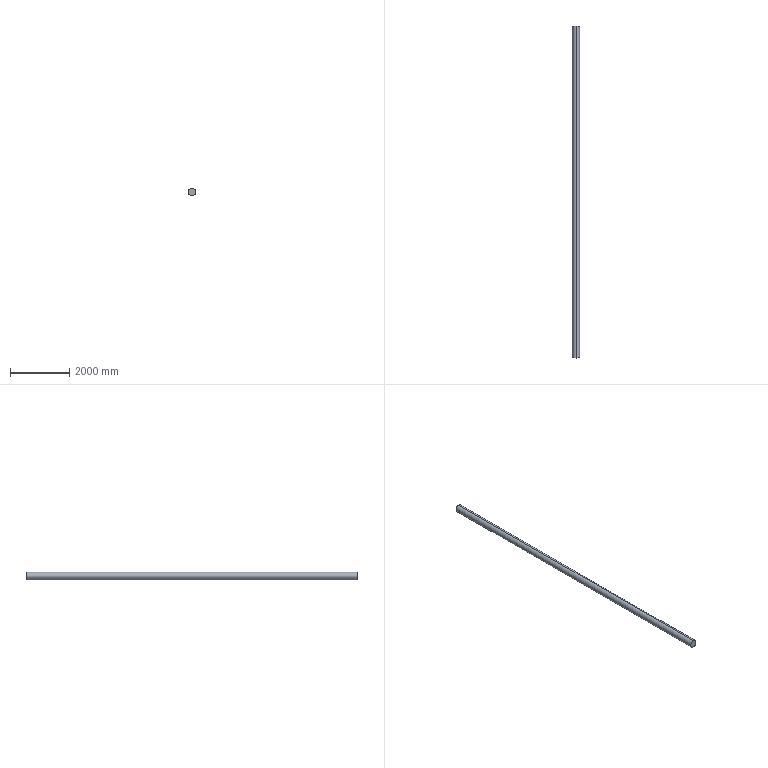Part | SolidWorks | features Extrusion 1 | 1 solid | 4 faces | box 250 x 11200 x 250 mm | volume 549778714 mm3 | cylinder 2 | plane 2 | commonest cylinder face diameters 250 x2
STEP:
#1=CARTESIAN_POINT('',(0.,11200.,125.));
#2=VERTEX_POINT('',#1);
#3=CARTESIAN_POINT('',(0.,11200.,-125.));
#4=VERTEX_POINT('',#3);
#5=CARTESIAN_POINT('',(0.,11200.,0.));
#6=DIRECTION('',(0.,1.,0.));
#7=DIRECTION('',(0.,0.,1.));
#8=AXIS2_PLACEMENT_3D('',#5,#6,#7);
#9=CIRCLE('',#8,125.);
#10=EDGE_CURVE('',#2,#4,#9,.T.);
#11=ORIENTED_EDGE('',*,*,#10,.F.);
#12=CARTESIAN_POINT('',(0.,0.,125.));
#13=VERTEX_POINT('',#12);
#14=CARTESIAN_POINT('',(0.,11200.,125.));
#15=DIRECTION('',(0.,-1.,0.));
#16=VECTOR('',#15,1000.);
#17=LINE('',#14,#16);
#18=EDGE_CURVE('',#2,#13,#17,.T.);
#19=ORIENTED_EDGE('',*,*,#18,.T.);
#20=CARTESIAN_POINT('',(0.,0.,-125.));
#21=VERTEX_POINT('',#20);
#22=CARTESIAN_POINT('',(0.,0.,0.));
#23=DIRECTION('',(0.,1.,0.));
#24=DIRECTION('',(0.,0.,1.));
#25=AXIS2_PLACEMENT_3D('',#22,#23,#24);
#26=CIRCLE('',#25,125.);
#27=EDGE_CURVE('',#13,#21,#26,.T.);
#28=ORIENTED_EDGE('',*,*,#27,.T.);
#29=CARTESIAN_POINT('',(0.,11200.,-125.));
#30=DIRECTION('',(0.,-1.,0.));
#31=VECTOR('',#30,1000.);
#32=LINE('',#29,#31);
#33=EDGE_CURVE('',#4,#21,#32,.T.);
#34=ORIENTED_EDGE('',*,*,#33,.F.);
#35=EDGE_LOOP('',(#11,#19,#28,#34));
#36=FACE_OUTER_BOUND('',#35,.T.);
#37=CARTESIAN_POINT('',(0.,11200.,0.));
#38=DIRECTION('',(0.,-1.,0.));
#39=DIRECTION('',(0.,0.,-1.));
#40=AXIS2_PLACEMENT_3D('',#37,#38,#39);
#41=CYLINDRICAL_SURFACE('',#40,125.);
#42=ADVANCED_FACE('',(#36),#41,.T.);
#43=ORIENTED_EDGE('',*,*,#18,.F.);
#44=CARTESIAN_POINT('',(0.,11200.,0.));
#45=DIRECTION('',(0.,1.,0.));
#46=DIRECTION('',(0.,0.,1.));
#47=AXIS2_PLACEMENT_3D('',#44,#45,#46);
#48=CIRCLE('',#47,125.);
#49=EDGE_CURVE('',#4,#2,#48,.T.);
#50=ORIENTED_EDGE('',*,*,#49,.F.);
#51=ORIENTED_EDGE('',*,*,#33,.T.);
#52=CARTESIAN_POINT('',(0.,0.,0.));
#53=DIRECTION('',(0.,1.,0.));
#54=DIRECTION('',(0.,0.,1.));
#55=AXIS2_PLACEMENT_3D('',#52,#53,#54);
#56=CIRCLE('',#55,125.);
#57=EDGE_CURVE('',#21,#13,#56,.T.);
#58=ORIENTED_EDGE('',*,*,#57,.T.);
#59=EDGE_LOOP('',(#43,#50,#51,#58));
#60=FACE_OUTER_BOUND('',#59,.T.);
#61=CARTESIAN_POINT('',(0.,11200.,0.));
#62=DIRECTION('',(0.,-1.,0.));
#63=DIRECTION('',(0.,0.,-1.));
#64=AXIS2_PLACEMENT_3D('',#61,#62,#63);
#65=CYLINDRICAL_SURFACE('',#64,125.);
#66=ADVANCED_FACE('',(#60),#65,.T.);
#67=ORIENTED_EDGE('',*,*,#49,.T.);
#68=ORIENTED_EDGE('',*,*,#10,.T.);
#69=EDGE_LOOP('',(#67,#68));
#70=FACE_OUTER_BOUND('',#69,.T.);
#71=CARTESIAN_POINT('',(0.,11200.,0.));
#72=DIRECTION('',(0.,1.,0.));
#73=DIRECTION('',(0.,0.,1.));
#74=AXIS2_PLACEMENT_3D('',#71,#72,#73);
#75=PLANE('',#74);
#76=ADVANCED_FACE('',(#70),#75,.T.);
#77=ORIENTED_EDGE('',*,*,#57,.F.);
#78=ORIENTED_EDGE('',*,*,#27,.F.);
#79=EDGE_LOOP('',(#77,#78));
#80=FACE_OUTER_BOUND('',#79,.T.);
#81=CARTESIAN_POINT('',(0.,0.,0.));
#82=DIRECTION('',(0.,1.,0.));
#83=DIRECTION('',(0.,0.,1.));
#84=AXIS2_PLACEMENT_3D('',#81,#82,#83);
#85=PLANE('',#84);
#86=ADVANCED_FACE('',(#80),#85,.F.);
#87=CLOSED_SHELL('',(#42,#66,#76,#86));
#88=MANIFOLD_SOLID_BREP('',#87);
#89=CARTESIAN_POINT('',(0.,0.,0.));
#90=DIRECTION('',(0.,0.,1.));
#91=DIRECTION('',(1.,0.,0.));
#92=AXIS2_PLACEMENT_3D('',#89,#90,#91);
#93=(LENGTH_UNIT()NAMED_UNIT(*)SI_UNIT(.MILLI.,.METRE.));
#94=UNCERTAINTY_MEASURE_WITH_UNIT(LENGTH_MEASURE(0.00001),#93,'','');
#95=(NAMED_UNIT(*)PLANE_ANGLE_UNIT()SI_UNIT($,.RADIAN.));
#96=(NAMED_UNIT(*)SI_UNIT($,.STERADIAN.)SOLID_ANGLE_UNIT());
#97=(GEOMETRIC_REPRESENTATION_CONTEXT(3)GLOBAL_UNCERTAINTY_ASSIGNED_CONTEXT((#94))GLOBAL_UNIT_ASSIGNED_CONTEXT((#93,#95,#96))REPRESENTATION_CONTEXT('',''));
#98=ADVANCED_BREP_SHAPE_REPRESENTATION('',(#88,#92),#97);